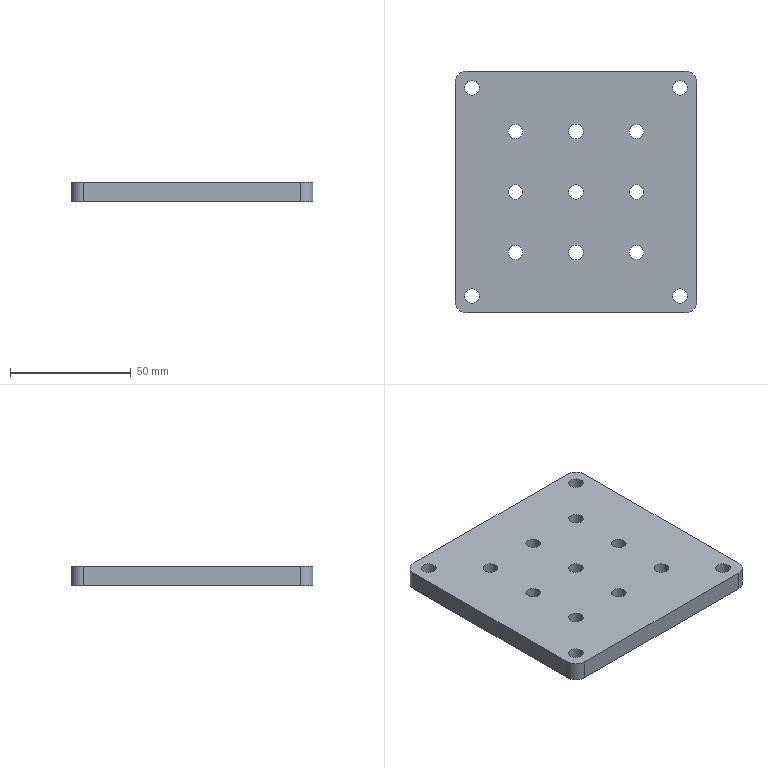Part | SolidWorks | features Extrusion 1 | 1 solid | 36 faces | box 100 x 100 x 8 mm | volume 76888 mm3 | cylinder 30 | plane 6 | commonest cylinder face diameters 6 x26 10 x4
STEP:
#1=CARTESIAN_POINT('',(-46.,-43.,8.));
#2=VERTEX_POINT('',#1);
#3=CARTESIAN_POINT('',(-40.,-43.,8.));
#4=VERTEX_POINT('',#3);
#5=CARTESIAN_POINT('',(-43.,-43.,8.));
#6=DIRECTION('',(0.,0.,1.));
#7=DIRECTION('',(1.,0.,0.));
#8=AXIS2_PLACEMENT_3D('',#5,#6,#7);
#9=CIRCLE('',#8,3.);
#10=EDGE_CURVE('',#2,#4,#9,.T.);
#11=ORIENTED_EDGE('',*,*,#10,.T.);
#12=CARTESIAN_POINT('',(-40.,-43.,0.));
#13=VERTEX_POINT('',#12);
#14=CARTESIAN_POINT('',(-40.,-43.,8.));
#15=DIRECTION('',(0.,0.,-1.));
#16=VECTOR('',#15,1000.);
#17=LINE('',#14,#16);
#18=EDGE_CURVE('',#4,#13,#17,.T.);
#19=ORIENTED_EDGE('',*,*,#18,.T.);
#20=CARTESIAN_POINT('',(-46.,-43.,0.));
#21=VERTEX_POINT('',#20);
#22=CARTESIAN_POINT('',(-43.,-43.,0.));
#23=DIRECTION('',(0.,0.,1.));
#24=DIRECTION('',(1.,0.,0.));
#25=AXIS2_PLACEMENT_3D('',#22,#23,#24);
#26=CIRCLE('',#25,3.);
#27=EDGE_CURVE('',#21,#13,#26,.T.);
#28=ORIENTED_EDGE('',*,*,#27,.F.);
#29=CARTESIAN_POINT('',(-46.,-43.,8.));
#30=DIRECTION('',(0.,0.,-1.));
#31=VECTOR('',#30,1000.);
#32=LINE('',#29,#31);
#33=EDGE_CURVE('',#2,#21,#32,.T.);
#34=ORIENTED_EDGE('',*,*,#33,.F.);
#35=EDGE_LOOP('',(#11,#19,#28,#34));
#36=FACE_OUTER_BOUND('',#35,.T.);
#37=CARTESIAN_POINT('',(-43.,-43.,8.));
#38=DIRECTION('',(0.,0.,-1.));
#39=DIRECTION('',(-1.,0.,0.));
#40=AXIS2_PLACEMENT_3D('',#37,#38,#39);
#41=CYLINDRICAL_SURFACE('',#40,3.);
#42=ADVANCED_FACE('',(#36),#41,.F.);
#43=CARTESIAN_POINT('',(40.,-43.,8.));
#44=VERTEX_POINT('',#43);
#45=CARTESIAN_POINT('',(46.,-43.,8.));
#46=VERTEX_POINT('',#45);
#47=CARTESIAN_POINT('',(43.,-43.,8.));
#48=DIRECTION('',(0.,0.,1.));
#49=DIRECTION('',(1.,0.,0.));
#50=AXIS2_PLACEMENT_3D('',#47,#48,#49);
#51=CIRCLE('',#50,3.);
#52=EDGE_CURVE('',#44,#46,#51,.T.);
#53=ORIENTED_EDGE('',*,*,#52,.T.);
#54=CARTESIAN_POINT('',(46.,-43.,0.));
#55=VERTEX_POINT('',#54);
#56=CARTESIAN_POINT('',(46.,-43.,8.));
#57=DIRECTION('',(0.,0.,-1.));
#58=VECTOR('',#57,1000.);
#59=LINE('',#56,#58);
#60=EDGE_CURVE('',#46,#55,#59,.T.);
#61=ORIENTED_EDGE('',*,*,#60,.T.);
#62=CARTESIAN_POINT('',(40.,-43.,0.));
#63=VERTEX_POINT('',#62);
#64=CARTESIAN_POINT('',(43.,-43.,0.));
#65=DIRECTION('',(0.,0.,1.));
#66=DIRECTION('',(1.,0.,0.));
#67=AXIS2_PLACEMENT_3D('',#64,#65,#66);
#68=CIRCLE('',#67,3.);
#69=EDGE_CURVE('',#63,#55,#68,.T.);
#70=ORIENTED_EDGE('',*,*,#69,.F.);
#71=CARTESIAN_POINT('',(40.,-43.,8.));
#72=DIRECTION('',(0.,0.,-1.));
#73=VECTOR('',#72,1000.);
#74=LINE('',#71,#73);
#75=EDGE_CURVE('',#44,#63,#74,.T.);
#76=ORIENTED_EDGE('',*,*,#75,.F.);
#77=EDGE_LOOP('',(#53,#61,#70,#76));
#78=FACE_OUTER_BOUND('',#77,.T.);
#79=CARTESIAN_POINT('',(43.,-43.,8.));
#80=DIRECTION('',(0.,0.,-1.));
#81=DIRECTION('',(-1.,0.,0.));
#82=AXIS2_PLACEMENT_3D('',#79,#80,#81);
#83=CYLINDRICAL_SURFACE('',#82,3.);
#84=ADVANCED_FACE('',(#78),#83,.F.);
#85=CARTESIAN_POINT('',(40.,43.,8.));
#86=VERTEX_POINT('',#85);
#87=CARTESIAN_POINT('',(46.,43.,8.));
#88=VERTEX_POINT('',#87);
#89=CARTESIAN_POINT('',(43.,43.,8.));
#90=DIRECTION('',(0.,0.,1.));
#91=DIRECTION('',(1.,0.,0.));
#92=AXIS2_PLACEMENT_3D('',#89,#90,#91);
#93=CIRCLE('',#92,3.);
#94=EDGE_CURVE('',#86,#88,#93,.T.);
#95=ORIENTED_EDGE('',*,*,#94,.T.);
#96=CARTESIAN_POINT('',(46.,43.,0.));
#97=VERTEX_POINT('',#96);
#98=CARTESIAN_POINT('',(46.,43.,8.));
#99=DIRECTION('',(0.,0.,-1.));
#100=VECTOR('',#99,1000.);
#101=LINE('',#98,#100);
#102=EDGE_CURVE('',#88,#97,#101,.T.);
#103=ORIENTED_EDGE('',*,*,#102,.T.);
#104=CARTESIAN_POINT('',(40.,43.,0.));
#105=VERTEX_POINT('',#104);
#106=CARTESIAN_POINT('',(43.,43.,0.));
#107=DIRECTION('',(0.,0.,1.));
#108=DIRECTION('',(1.,0.,0.));
#109=AXIS2_PLACEMENT_3D('',#106,#107,#108);
#110=CIRCLE('',#109,3.);
#111=EDGE_CURVE('',#105,#97,#110,.T.);
#112=ORIENTED_EDGE('',*,*,#111,.F.);
#113=CARTESIAN_POINT('',(40.,43.,8.));
#114=DIRECTION('',(0.,0.,-1.));
#115=VECTOR('',#114,1000.);
#116=LINE('',#113,#115);
#117=EDGE_CURVE('',#86,#105,#116,.T.);
#118=ORIENTED_EDGE('',*,*,#117,.F.);
#119=EDGE_LOOP('',(#95,#103,#112,#118));
#120=FACE_OUTER_BOUND('',#119,.T.);
#121=CARTESIAN_POINT('',(43.,43.,8.));
#122=DIRECTION('',(0.,0.,-1.));
#123=DIRECTION('',(-1.,0.,0.));
#124=AXIS2_PLACEMENT_3D('',#121,#122,#123);
#125=CYLINDRICAL_SURFACE('',#124,3.);
#126=ADVANCED_FACE('',(#120),#125,.F.);
#127=CARTESIAN_POINT('',(-46.,43.,8.));
#128=VERTEX_POINT('',#127);
#129=CARTESIAN_POINT('',(-40.,43.,8.));
#130=VERTEX_POINT('',#129);
#131=CARTESIAN_POINT('',(-43.,43.,8.));
#132=DIRECTION('',(0.,0.,1.));
#133=DIRECTION('',(1.,0.,0.));
#134=AXIS2_PLACEMENT_3D('',#131,#132,#133);
#135=CIRCLE('',#134,3.);
#136=EDGE_CURVE('',#128,#130,#135,.T.);
#137=ORIENTED_EDGE('',*,*,#136,.T.);
#138=CARTESIAN_POINT('',(-40.,43.,0.));
#139=VERTEX_POINT('',#138);
#140=CARTESIAN_POINT('',(-40.,43.,8.));
#141=DIRECTION('',(0.,0.,-1.));
#142=VECTOR('',#141,1000.);
#143=LINE('',#140,#142);
#144=EDGE_CURVE('',#130,#139,#143,.T.);
#145=ORIENTED_EDGE('',*,*,#144,.T.);
#146=CARTESIAN_POINT('',(-46.,43.,0.));
#147=VERTEX_POINT('',#146);
#148=CARTESIAN_POINT('',(-43.,43.,0.));
#149=DIRECTION('',(0.,0.,1.));
#150=DIRECTION('',(1.,0.,0.));
#151=AXIS2_PLACEMENT_3D('',#148,#149,#150);
#152=CIRCLE('',#151,3.);
#153=EDGE_CURVE('',#147,#139,#152,.T.);
#154=ORIENTED_EDGE('',*,*,#153,.F.);
#155=CARTESIAN_POINT('',(-46.,43.,8.));
#156=DIRECTION('',(0.,0.,-1.));
#157=VECTOR('',#156,1000.);
#158=LINE('',#155,#157);
#159=EDGE_CURVE('',#128,#147,#158,.T.);
#160=ORIENTED_EDGE('',*,*,#159,.F.);
#161=EDGE_LOOP('',(#137,#145,#154,#160));
#162=FACE_OUTER_BOUND('',#161,.T.);
#163=CARTESIAN_POINT('',(-43.,43.,8.));
#164=DIRECTION('',(0.,0.,-1.));
#165=DIRECTION('',(-1.,0.,0.));
#166=AXIS2_PLACEMENT_3D('',#163,#164,#165);
#167=CYLINDRICAL_SURFACE('',#166,3.);
#168=ADVANCED_FACE('',(#162),#167,.F.);
#169=CARTESIAN_POINT('',(-28.,-25.,8.));
#170=VERTEX_POINT('',#169);
#171=CARTESIAN_POINT('',(-22.,-25.,8.));
#172=VERTEX_POINT('',#171);
#173=CARTESIAN_POINT('',(-25.,-25.,8.));
#174=DIRECTION('',(0.,0.,1.));
#175=DIRECTION('',(1.,0.,0.));
#176=AXIS2_PLACEMENT_3D('',#173,#174,#175);
#177=CIRCLE('',#176,3.);
#178=EDGE_CURVE('',#170,#172,#177,.T.);
#179=ORIENTED_EDGE('',*,*,#178,.T.);
#180=CARTESIAN_POINT('',(-22.,-25.,0.));
#181=VERTEX_POINT('',#180);
#182=CARTESIAN_POINT('',(-22.,-25.,8.));
#183=DIRECTION('',(0.,0.,-1.));
#184=VECTOR('',#183,1000.);
#185=LINE('',#182,#184);
#186=EDGE_CURVE('',#172,#181,#185,.T.);
#187=ORIENTED_EDGE('',*,*,#186,.T.);
#188=CARTESIAN_POINT('',(-28.,-25.,0.));
#189=VERTEX_POINT('',#188);
#190=CARTESIAN_POINT('',(-25.,-25.,0.));
#191=DIRECTION('',(0.,0.,1.));
#192=DIRECTION('',(1.,0.,0.));
#193=AXIS2_PLACEMENT_3D('',#190,#191,#192);
#194=CIRCLE('',#193,3.);
#195=EDGE_CURVE('',#189,#181,#194,.T.);
#196=ORIENTED_EDGE('',*,*,#195,.F.);
#197=CARTESIAN_POINT('',(-28.,-25.,8.));
#198=DIRECTION('',(0.,0.,-1.));
#199=VECTOR('',#198,1000.);
#200=LINE('',#197,#199);
#201=EDGE_CURVE('',#170,#189,#200,.T.);
#202=ORIENTED_EDGE('',*,*,#201,.F.);
#203=EDGE_LOOP('',(#179,#187,#196,#202));
#204=FACE_OUTER_BOUND('',#203,.T.);
#205=CARTESIAN_POINT('',(-25.,-25.,8.));
#206=DIRECTION('',(0.,0.,-1.));
#207=DIRECTION('',(-1.,0.,0.));
#208=AXIS2_PLACEMENT_3D('',#205,#206,#207);
#209=CYLINDRICAL_SURFACE('',#208,3.);
#210=ADVANCED_FACE('',(#204),#209,.F.);
#211=CARTESIAN_POINT('',(-28.,0.,8.));
#212=VERTEX_POINT('',#211);
#213=CARTESIAN_POINT('',(-22.,0.,8.));
#214=VERTEX_POINT('',#213);
#215=CARTESIAN_POINT('',(-25.,0.,8.));
#216=DIRECTION('',(0.,0.,1.));
#217=DIRECTION('',(1.,0.,0.));
#218=AXIS2_PLACEMENT_3D('',#215,#216,#217);
#219=CIRCLE('',#218,3.);
#220=EDGE_CURVE('',#212,#214,#219,.T.);
#221=ORIENTED_EDGE('',*,*,#220,.T.);
#222=CARTESIAN_POINT('',(-22.,0.,0.));
#223=VERTEX_POINT('',#222);
#224=CARTESIAN_POINT('',(-22.,0.,8.));
#225=DIRECTION('',(0.,0.,-1.));
#226=VECTOR('',#225,1000.);
#227=LINE('',#224,#226);
#228=EDGE_CURVE('',#214,#223,#227,.T.);
#229=ORIENTED_EDGE('',*,*,#228,.T.);
#230=CARTESIAN_POINT('',(-28.,0.,0.));
#231=VERTEX_POINT('',#230);
#232=CARTESIAN_POINT('',(-25.,0.,0.));
#233=DIRECTION('',(0.,0.,1.));
#234=DIRECTION('',(1.,0.,0.));
#235=AXIS2_PLACEMENT_3D('',#232,#233,#234);
#236=CIRCLE('',#235,3.);
#237=EDGE_CURVE('',#231,#223,#236,.T.);
#238=ORIENTED_EDGE('',*,*,#237,.F.);
#239=CARTESIAN_POINT('',(-28.,0.,8.));
#240=DIRECTION('',(0.,0.,-1.));
#241=VECTOR('',#240,1000.);
#242=LINE('',#239,#241);
#243=EDGE_CURVE('',#212,#231,#242,.T.);
#244=ORIENTED_EDGE('',*,*,#243,.F.);
#245=EDGE_LOOP('',(#221,#229,#238,#244));
#246=FACE_OUTER_BOUND('',#245,.T.);
#247=CARTESIAN_POINT('',(-25.,0.,8.));
#248=DIRECTION('',(0.,0.,-1.));
#249=DIRECTION('',(-1.,0.,0.));
#250=AXIS2_PLACEMENT_3D('',#247,#248,#249);
#251=CYLINDRICAL_SURFACE('',#250,3.);
#252=ADVANCED_FACE('',(#246),#251,.F.);
#253=CARTESIAN_POINT('',(22.,-25.,8.));
#254=VERTEX_POINT('',#253);
#255=CARTESIAN_POINT('',(28.,-25.,8.));
#256=VERTEX_POINT('',#255);
#257=CARTESIAN_POINT('',(25.,-25.,8.));
#258=DIRECTION('',(0.,0.,1.));
#259=DIRECTION('',(1.,0.,0.));
#260=AXIS2_PLACEMENT_3D('',#257,#258,#259);
#261=CIRCLE('',#260,3.);
#262=EDGE_CURVE('',#254,#256,#261,.T.);
#263=ORIENTED_EDGE('',*,*,#262,.T.);
#264=CARTESIAN_POINT('',(28.,-25.,0.));
#265=VERTEX_POINT('',#264);
#266=CARTESIAN_POINT('',(28.,-25.,8.));
#267=DIRECTION('',(0.,0.,-1.));
#268=VECTOR('',#267,1000.);
#269=LINE('',#266,#268);
#270=EDGE_CURVE('',#256,#265,#269,.T.);
#271=ORIENTED_EDGE('',*,*,#270,.T.);
#272=CARTESIAN_POINT('',(22.,-25.,0.));
#273=VERTEX_POINT('',#272);
#274=CARTESIAN_POINT('',(25.,-25.,0.));
#275=DIRECTION('',(0.,0.,1.));
#276=DIRECTION('',(1.,0.,0.));
#277=AXIS2_PLACEMENT_3D('',#274,#275,#276);
#278=CIRCLE('',#277,3.);
#279=EDGE_CURVE('',#273,#265,#278,.T.);
#280=ORIENTED_EDGE('',*,*,#279,.F.);
#281=CARTESIAN_POINT('',(22.,-25.,8.));
#282=DIRECTION('',(0.,0.,-1.));
#283=VECTOR('',#282,1000.);
#284=LINE('',#281,#283);
#285=EDGE_CURVE('',#254,#273,#284,.T.);
#286=ORIENTED_EDGE('',*,*,#285,.F.);
#287=EDGE_LOOP('',(#263,#271,#280,#286));
#288=FACE_OUTER_BOUND('',#287,.T.);
#289=CARTESIAN_POINT('',(25.,-25.,8.));
#290=DIRECTION('',(0.,0.,-1.));
#291=DIRECTION('',(-1.,0.,0.));
#292=AXIS2_PLACEMENT_3D('',#289,#290,#291);
#293=CYLINDRICAL_SURFACE('',#292,3.);
#294=ADVANCED_FACE('',(#288),#293,.F.);
#295=CARTESIAN_POINT('',(-3.,-25.,8.));
#296=VERTEX_POINT('',#295);
#297=CARTESIAN_POINT('',(3.,-25.,8.));
#298=VERTEX_POINT('',#297);
#299=CARTESIAN_POINT('',(0.,-25.,8.));
#300=DIRECTION('',(0.,0.,1.));
#301=DIRECTION('',(1.,0.,0.));
#302=AXIS2_PLACEMENT_3D('',#299,#300,#301);
#303=CIRCLE('',#302,3.);
#304=EDGE_CURVE('',#296,#298,#303,.T.);
#305=ORIENTED_EDGE('',*,*,#304,.T.);
#306=CARTESIAN_POINT('',(3.,-25.,0.));
#307=VERTEX_POINT('',#306);
#308=CARTESIAN_POINT('',(3.,-25.,8.));
#309=DIRECTION('',(0.,0.,-1.));
#310=VECTOR('',#309,1000.);
#311=LINE('',#308,#310);
#312=EDGE_CURVE('',#298,#307,#311,.T.);
#313=ORIENTED_EDGE('',*,*,#312,.T.);
#314=CARTESIAN_POINT('',(-3.,-25.,0.));
#315=VERTEX_POINT('',#314);
#316=CARTESIAN_POINT('',(0.,-25.,0.));
#317=DIRECTION('',(0.,0.,1.));
#318=DIRECTION('',(1.,0.,0.));
#319=AXIS2_PLACEMENT_3D('',#316,#317,#318);
#320=CIRCLE('',#319,3.);
#321=EDGE_CURVE('',#315,#307,#320,.T.);
#322=ORIENTED_EDGE('',*,*,#321,.F.);
#323=CARTESIAN_POINT('',(-3.,-25.,8.));
#324=DIRECTION('',(0.,0.,-1.));
#325=VECTOR('',#324,1000.);
#326=LINE('',#323,#325);
#327=EDGE_CURVE('',#296,#315,#326,.T.);
#328=ORIENTED_EDGE('',*,*,#327,.F.);
#329=EDGE_LOOP('',(#305,#313,#322,#328));
#330=FACE_OUTER_BOUND('',#329,.T.);
#331=CARTESIAN_POINT('',(0.,-25.,8.));
#332=DIRECTION('',(0.,0.,-1.));
#333=DIRECTION('',(-1.,0.,0.));
#334=AXIS2_PLACEMENT_3D('',#331,#332,#333);
#335=CYLINDRICAL_SURFACE('',#334,3.);
#336=ADVANCED_FACE('',(#330),#335,.F.);
#337=CARTESIAN_POINT('',(22.,0.,8.));
#338=VERTEX_POINT('',#337);
#339=CARTESIAN_POINT('',(28.,0.,8.));
#340=VERTEX_POINT('',#339);
#341=CARTESIAN_POINT('',(25.,0.,8.));
#342=DIRECTION('',(0.,0.,1.));
#343=DIRECTION('',(1.,0.,0.));
#344=AXIS2_PLACEMENT_3D('',#341,#342,#343);
#345=CIRCLE('',#344,3.);
#346=EDGE_CURVE('',#338,#340,#345,.T.);
#347=ORIENTED_EDGE('',*,*,#346,.T.);
#348=CARTESIAN_POINT('',(28.,0.,0.));
#349=VERTEX_POINT('',#348);
#350=CARTESIAN_POINT('',(28.,0.,8.));
#351=DIRECTION('',(0.,0.,-1.));
#352=VECTOR('',#351,1000.);
#353=LINE('',#350,#352);
#354=EDGE_CURVE('',#340,#349,#353,.T.);
#355=ORIENTED_EDGE('',*,*,#354,.T.);
#356=CARTESIAN_POINT('',(22.,0.,0.));
#357=VERTEX_POINT('',#356);
#358=CARTESIAN_POINT('',(25.,0.,0.));
#359=DIRECTION('',(0.,0.,1.));
#360=DIRECTION('',(1.,0.,0.));
#361=AXIS2_PLACEMENT_3D('',#358,#359,#360);
#362=CIRCLE('',#361,3.);
#363=EDGE_CURVE('',#357,#349,#362,.T.);
#364=ORIENTED_EDGE('',*,*,#363,.F.);
#365=CARTESIAN_POINT('',(22.,0.,8.));
#366=DIRECTION('',(0.,0.,-1.));
#367=VECTOR('',#366,1000.);
#368=LINE('',#365,#367);
#369=EDGE_CURVE('',#338,#357,#368,.T.);
#370=ORIENTED_EDGE('',*,*,#369,.F.);
#371=EDGE_LOOP('',(#347,#355,#364,#370));
#372=FACE_OUTER_BOUND('',#371,.T.);
#373=CARTESIAN_POINT('',(25.,0.,8.));
#374=DIRECTION('',(0.,0.,-1.));
#375=DIRECTION('',(-1.,0.,0.));
#376=AXIS2_PLACEMENT_3D('',#373,#374,#375);
#377=CYLINDRICAL_SURFACE('',#376,3.);
#378=ADVANCED_FACE('',(#372),#377,.F.);
#379=CARTESIAN_POINT('',(-3.,0.,8.));
#380=VERTEX_POINT('',#379);
#381=CARTESIAN_POINT('',(3.,0.,8.));
#382=VERTEX_POINT('',#381);
#383=CARTESIAN_POINT('',(0.,0.,8.));
#384=DIRECTION('',(0.,0.,1.));
#385=DIRECTION('',(1.,0.,0.));
#386=AXIS2_PLACEMENT_3D('',#383,#384,#385);
#387=CIRCLE('',#386,3.);
#388=EDGE_CURVE('',#380,#382,#387,.T.);
#389=ORIENTED_EDGE('',*,*,#388,.T.);
#390=CARTESIAN_POINT('',(3.,0.,0.));
#391=VERTEX_POINT('',#390);
#392=CARTESIAN_POINT('',(3.,0.,8.));
#393=DIRECTION('',(0.,0.,-1.));
#394=VECTOR('',#393,1000.);
#395=LINE('',#392,#394);
#396=EDGE_CURVE('',#382,#391,#395,.T.);
#397=ORIENTED_EDGE('',*,*,#396,.T.);
#398=CARTESIAN_POINT('',(-3.,0.,0.));
#399=VERTEX_POINT('',#398);
#400=CARTESIAN_POINT('',(0.,0.,0.));
#401=DIRECTION('',(0.,0.,1.));
#402=DIRECTION('',(1.,0.,0.));
#403=AXIS2_PLACEMENT_3D('',#400,#401,#402);
#404=CIRCLE('',#403,3.);
#405=EDGE_CURVE('',#399,#391,#404,.T.);
#406=ORIENTED_EDGE('',*,*,#405,.F.);
#407=CARTESIAN_POINT('',(-3.,0.,8.));
#408=DIRECTION('',(0.,0.,-1.));
#409=VECTOR('',#408,1000.);
#410=LINE('',#407,#409);
#411=EDGE_CURVE('',#380,#399,#410,.T.);
#412=ORIENTED_EDGE('',*,*,#411,.F.);
#413=EDGE_LOOP('',(#389,#397,#406,#412));
#414=FACE_OUTER_BOUND('',#413,.T.);
#415=CARTESIAN_POINT('',(0.,0.,8.));
#416=DIRECTION('',(0.,0.,-1.));
#417=DIRECTION('',(-1.,0.,0.));
#418=AXIS2_PLACEMENT_3D('',#415,#416,#417);
#419=CYLINDRICAL_SURFACE('',#418,3.);
#420=ADVANCED_FACE('',(#414),#419,.F.);
#421=CARTESIAN_POINT('',(22.,25.,8.));
#422=VERTEX_POINT('',#421);
#423=CARTESIAN_POINT('',(28.,25.,8.));
#424=VERTEX_POINT('',#423);
#425=CARTESIAN_POINT('',(25.,25.,8.));
#426=DIRECTION('',(0.,0.,1.));
#427=DIRECTION('',(1.,0.,0.));
#428=AXIS2_PLACEMENT_3D('',#425,#426,#427);
#429=CIRCLE('',#428,3.);
#430=EDGE_CURVE('',#422,#424,#429,.T.);
#431=ORIENTED_EDGE('',*,*,#430,.T.);
#432=CARTESIAN_POINT('',(28.,25.,0.));
#433=VERTEX_POINT('',#432);
#434=CARTESIAN_POINT('',(28.,25.,8.));
#435=DIRECTION('',(0.,0.,-1.));
#436=VECTOR('',#435,1000.);
#437=LINE('',#434,#436);
#438=EDGE_CURVE('',#424,#433,#437,.T.);
#439=ORIENTED_EDGE('',*,*,#438,.T.);
#440=CARTESIAN_POINT('',(22.,25.,0.));
#441=VERTEX_POINT('',#440);
#442=CARTESIAN_POINT('',(25.,25.,0.));
#443=DIRECTION('',(0.,0.,1.));
#444=DIRECTION('',(1.,0.,0.));
#445=AXIS2_PLACEMENT_3D('',#442,#443,#444);
#446=CIRCLE('',#445,3.);
#447=EDGE_CURVE('',#441,#433,#446,.T.);
#448=ORIENTED_EDGE('',*,*,#447,.F.);
#449=CARTESIAN_POINT('',(22.,25.,8.));
#450=DIRECTION('',(0.,0.,-1.));
#451=VECTOR('',#450,1000.);
#452=LINE('',#449,#451);
#453=EDGE_CURVE('',#422,#441,#452,.T.);
#454=ORIENTED_EDGE('',*,*,#453,.F.);
#455=EDGE_LOOP('',(#431,#439,#448,#454));
#456=FACE_OUTER_BOUND('',#455,.T.);
#457=CARTESIAN_POINT('',(25.,25.,8.));
#458=DIRECTION('',(0.,0.,-1.));
#459=DIRECTION('',(-1.,0.,0.));
#460=AXIS2_PLACEMENT_3D('',#457,#458,#459);
#461=CYLINDRICAL_SURFACE('',#460,3.);
#462=ADVANCED_FACE('',(#456),#461,.F.);
#463=CARTESIAN_POINT('',(-3.,25.,8.));
#464=VERTEX_POINT('',#463);
#465=CARTESIAN_POINT('',(3.,25.,8.));
#466=VERTEX_POINT('',#465);
#467=CARTESIAN_POINT('',(0.,25.,8.));
#468=DIRECTION('',(0.,0.,1.));
#469=DIRECTION('',(1.,0.,0.));
#470=AXIS2_PLACEMENT_3D('',#467,#468,#469);
#471=CIRCLE('',#470,3.);
#472=EDGE_CURVE('',#464,#466,#471,.T.);
#473=ORIENTED_EDGE('',*,*,#472,.T.);
#474=CARTESIAN_POINT('',(3.,25.,0.));
#475=VERTEX_POINT('',#474);
#476=CARTESIAN_POINT('',(3.,25.,8.));
#477=DIRECTION('',(0.,0.,-1.));
#478=VECTOR('',#477,1000.);
#479=LINE('',#476,#478);
#480=EDGE_CURVE('',#466,#475,#479,.T.);
#481=ORIENTED_EDGE('',*,*,#480,.T.);
#482=CARTESIAN_POINT('',(-3.,25.,0.));
#483=VERTEX_POINT('',#482);
#484=CARTESIAN_POINT('',(0.,25.,0.));
#485=DIRECTION('',(0.,0.,1.));
#486=DIRECTION('',(1.,0.,0.));
#487=AXIS2_PLACEMENT_3D('',#484,#485,#486);
#488=CIRCLE('',#487,3.);
#489=EDGE_CURVE('',#483,#475,#488,.T.);
#490=ORIENTED_EDGE('',*,*,#489,.F.);
#491=CARTESIAN_POINT('',(-3.,25.,8.));
#492=DIRECTION('',(0.,0.,-1.));
#493=VECTOR('',#492,1000.);
#494=LINE('',#491,#493);
#495=EDGE_CURVE('',#464,#483,#494,.T.);
#496=ORIENTED_EDGE('',*,*,#495,.F.);
#497=EDGE_LOOP('',(#473,#481,#490,#496));
#498=FACE_OUTER_BOUND('',#497,.T.);
#499=CARTESIAN_POINT('',(0.,25.,8.));
#500=DIRECTION('',(0.,0.,-1.));
#501=DIRECTION('',(-1.,0.,0.));
#502=AXIS2_PLACEMENT_3D('',#499,#500,#501);
#503=CYLINDRICAL_SURFACE('',#502,3.);
#504=ADVANCED_FACE('',(#498),#503,.F.);
#505=CARTESIAN_POINT('',(-28.,25.,8.));
#506=VERTEX_POINT('',#505);
#507=CARTESIAN_POINT('',(-22.,25.,8.));
#508=VERTEX_POINT('',#507);
#509=CARTESIAN_POINT('',(-25.,25.,8.));
#510=DIRECTION('',(0.,0.,1.));
#511=DIRECTION('',(1.,0.,0.));
#512=AXIS2_PLACEMENT_3D('',#509,#510,#511);
#513=CIRCLE('',#512,3.);
#514=EDGE_CURVE('',#506,#508,#513,.T.);
#515=ORIENTED_EDGE('',*,*,#514,.T.);
#516=CARTESIAN_POINT('',(-22.,25.,0.));
#517=VERTEX_POINT('',#516);
#518=CARTESIAN_POINT('',(-22.,25.,8.));
#519=DIRECTION('',(0.,0.,-1.));
#520=VECTOR('',#519,1000.);
#521=LINE('',#518,#520);
#522=EDGE_CURVE('',#508,#517,#521,.T.);
#523=ORIENTED_EDGE('',*,*,#522,.T.);
#524=CARTESIAN_POINT('',(-28.,25.,0.));
#525=VERTEX_POINT('',#524);
#526=CARTESIAN_POINT('',(-25.,25.,0.));
#527=DIRECTION('',(0.,0.,1.));
#528=DIRECTION('',(1.,0.,0.));
#529=AXIS2_PLACEMENT_3D('',#526,#527,#528);
#530=CIRCLE('',#529,3.);
#531=EDGE_CURVE('',#525,#517,#530,.T.);
#532=ORIENTED_EDGE('',*,*,#531,.F.);
#533=CARTESIAN_POINT('',(-28.,25.,8.));
#534=DIRECTION('',(0.,0.,-1.));
#535=VECTOR('',#534,1000.);
#536=LINE('',#533,#535);
#537=EDGE_CURVE('',#506,#525,#536,.T.);
#538=ORIENTED_EDGE('',*,*,#537,.F.);
#539=EDGE_LOOP('',(#515,#523,#532,#538));
#540=FACE_OUTER_BOUND('',#539,.T.);
#541=CARTESIAN_POINT('',(-25.,25.,8.));
#542=DIRECTION('',(0.,0.,-1.));
#543=DIRECTION('',(-1.,0.,0.));
#544=AXIS2_PLACEMENT_3D('',#541,#542,#543);
#545=CYLINDRICAL_SURFACE('',#544,3.);
#546=ADVANCED_FACE('',(#540),#545,.F.);
#547=ORIENTED_EDGE('',*,*,#52,.F.);
#548=CARTESIAN_POINT('',(43.,-43.,8.));
#549=DIRECTION('',(0.,0.,1.));
#550=DIRECTION('',(1.,0.,0.));
#551=AXIS2_PLACEMENT_3D('',#548,#549,#550);
#552=CIRCLE('',#551,3.);
#553=EDGE_CURVE('',#46,#44,#552,.T.);
#554=ORIENTED_EDGE('',*,*,#553,.F.);
#555=EDGE_LOOP('',(#547,#554));
#556=FACE_BOUND('',#555,.T.);
#557=ORIENTED_EDGE('',*,*,#136,.F.);
#558=CARTESIAN_POINT('',(-43.,43.,8.));
#559=DIRECTION('',(0.,0.,1.));
#560=DIRECTION('',(1.,0.,0.));
#561=AXIS2_PLACEMENT_3D('',#558,#559,#560);
#562=CIRCLE('',#561,3.);
#563=EDGE_CURVE('',#130,#128,#562,.T.);
#564=ORIENTED_EDGE('',*,*,#563,.F.);
#565=EDGE_LOOP('',(#557,#564));
#566=FACE_BOUND('',#565,.T.);
#567=ORIENTED_EDGE('',*,*,#220,.F.);
#568=CARTESIAN_POINT('',(-25.,0.,8.));
#569=DIRECTION('',(0.,0.,1.));
#570=DIRECTION('',(1.,0.,0.));
#571=AXIS2_PLACEMENT_3D('',#568,#569,#570);
#572=CIRCLE('',#571,3.);
#573=EDGE_CURVE('',#214,#212,#572,.T.);
#574=ORIENTED_EDGE('',*,*,#573,.F.);
#575=EDGE_LOOP('',(#567,#574));
#576=FACE_BOUND('',#575,.T.);
#577=ORIENTED_EDGE('',*,*,#304,.F.);
#578=CARTESIAN_POINT('',(0.,-25.,8.));
#579=DIRECTION('',(0.,0.,1.));
#580=DIRECTION('',(1.,0.,0.));
#581=AXIS2_PLACEMENT_3D('',#578,#579,#580);
#582=CIRCLE('',#581,3.);
#583=EDGE_CURVE('',#298,#296,#582,.T.);
#584=ORIENTED_EDGE('',*,*,#583,.F.);
#585=EDGE_LOOP('',(#577,#584));
#586=FACE_BOUND('',#585,.T.);
#587=ORIENTED_EDGE('',*,*,#388,.F.);
#588=CARTESIAN_POINT('',(0.,0.,8.));
#589=DIRECTION('',(0.,0.,1.));
#590=DIRECTION('',(1.,0.,0.));
#591=AXIS2_PLACEMENT_3D('',#588,#589,#590);
#592=CIRCLE('',#591,3.);
#593=EDGE_CURVE('',#382,#380,#592,.T.);
#594=ORIENTED_EDGE('',*,*,#593,.F.);
#595=EDGE_LOOP('',(#587,#594));
#596=FACE_BOUND('',#595,.T.);
#597=ORIENTED_EDGE('',*,*,#472,.F.);
#598=CARTESIAN_POINT('',(0.,25.,8.));
#599=DIRECTION('',(0.,0.,1.));
#600=DIRECTION('',(1.,0.,0.));
#601=AXIS2_PLACEMENT_3D('',#598,#599,#600);
#602=CIRCLE('',#601,3.);
#603=EDGE_CURVE('',#466,#464,#602,.T.);
#604=ORIENTED_EDGE('',*,*,#603,.F.);
#605=EDGE_LOOP('',(#597,#604));
#606=FACE_BOUND('',#605,.T.);
#607=CARTESIAN_POINT('',(45.,-50.,8.));
#608=VERTEX_POINT('',#607);
#609=CARTESIAN_POINT('',(50.,-45.,8.));
#610=VERTEX_POINT('',#609);
#611=CARTESIAN_POINT('',(45.,-45.,8.));
#612=DIRECTION('',(0.,0.,1.));
#613=DIRECTION('',(1.,0.,0.));
#614=AXIS2_PLACEMENT_3D('',#611,#612,#613);
#615=CIRCLE('',#614,5.);
#616=EDGE_CURVE('',#608,#610,#615,.T.);
#617=ORIENTED_EDGE('',*,*,#616,.T.);
#618=CARTESIAN_POINT('',(50.,45.,8.));
#619=VERTEX_POINT('',#618);
#620=CARTESIAN_POINT('',(50.,45.,8.));
#621=DIRECTION('',(0.,1.,0.));
#622=VECTOR('',#621,1000.);
#623=LINE('',#620,#622);
#624=EDGE_CURVE('',#610,#619,#623,.T.);
#625=ORIENTED_EDGE('',*,*,#624,.T.);
#626=CARTESIAN_POINT('',(45.,50.,8.));
#627=VERTEX_POINT('',#626);
#628=CARTESIAN_POINT('',(45.,45.,8.));
#629=DIRECTION('',(0.,0.,1.));
#630=DIRECTION('',(-1.,0.,0.));
#631=AXIS2_PLACEMENT_3D('',#628,#629,#630);
#632=CIRCLE('',#631,5.);
#633=EDGE_CURVE('',#619,#627,#632,.T.);
#634=ORIENTED_EDGE('',*,*,#633,.T.);
#635=CARTESIAN_POINT('',(-45.,50.,8.));
#636=VERTEX_POINT('',#635);
#637=CARTESIAN_POINT('',(-45.,50.,8.));
#638=DIRECTION('',(-1.,0.,0.));
#639=VECTOR('',#638,1000.);
#640=LINE('',#637,#639);
#641=EDGE_CURVE('',#627,#636,#640,.T.);
#642=ORIENTED_EDGE('',*,*,#641,.T.);
#643=CARTESIAN_POINT('',(-50.,45.,8.));
#644=VERTEX_POINT('',#643);
#645=CARTESIAN_POINT('',(-45.,45.,8.));
#646=DIRECTION('',(0.,0.,1.));
#647=DIRECTION('',(1.,0.,0.));
#648=AXIS2_PLACEMENT_3D('',#645,#646,#647);
#649=CIRCLE('',#648,5.);
#650=EDGE_CURVE('',#636,#644,#649,.T.);
#651=ORIENTED_EDGE('',*,*,#650,.T.);
#652=CARTESIAN_POINT('',(-50.,-45.,8.));
#653=VERTEX_POINT('',#652);
#654=CARTESIAN_POINT('',(-50.,45.,8.));
#655=DIRECTION('',(0.,-1.,0.));
#656=VECTOR('',#655,1000.);
#657=LINE('',#654,#656);
#658=EDGE_CURVE('',#644,#653,#657,.T.);
#659=ORIENTED_EDGE('',*,*,#658,.T.);
#660=CARTESIAN_POINT('',(-45.,-50.,8.));
#661=VERTEX_POINT('',#660);
#662=CARTESIAN_POINT('',(-45.,-45.,8.));
#663=DIRECTION('',(0.,0.,1.));
#664=DIRECTION('',(1.,0.,0.));
#665=AXIS2_PLACEMENT_3D('',#662,#663,#664);
#666=CIRCLE('',#665,5.);
#667=EDGE_CURVE('',#653,#661,#666,.T.);
#668=ORIENTED_EDGE('',*,*,#667,.T.);
#669=CARTESIAN_POINT('',(-45.,-50.,8.));
#670=DIRECTION('',(1.,0.,0.));
#671=VECTOR('',#670,1000.);
#672=LINE('',#669,#671);
#673=EDGE_CURVE('',#661,#608,#672,.T.);
#674=ORIENTED_EDGE('',*,*,#673,.T.);
#675=EDGE_LOOP('',(#617,#625,#634,#642,#651,#659,#668,#674));
#676=FACE_OUTER_BOUND('',#675,.T.);
#677=ORIENTED_EDGE('',*,*,#514,.F.);
#678=CARTESIAN_POINT('',(-25.,25.,8.));
#679=DIRECTION('',(0.,0.,1.));
#680=DIRECTION('',(1.,0.,0.));
#681=AXIS2_PLACEMENT_3D('',#678,#679,#680);
#682=CIRCLE('',#681,3.);
#683=EDGE_CURVE('',#508,#506,#682,.T.);
#684=ORIENTED_EDGE('',*,*,#683,.F.);
#685=EDGE_LOOP('',(#677,#684));
#686=FACE_BOUND('',#685,.T.);
#687=ORIENTED_EDGE('',*,*,#430,.F.);
#688=CARTESIAN_POINT('',(25.,25.,8.));
#689=DIRECTION('',(0.,0.,1.));
#690=DIRECTION('',(1.,0.,0.));
#691=AXIS2_PLACEMENT_3D('',#688,#689,#690);
#692=CIRCLE('',#691,3.);
#693=EDGE_CURVE('',#424,#422,#692,.T.);
#694=ORIENTED_EDGE('',*,*,#693,.F.);
#695=EDGE_LOOP('',(#687,#694));
#696=FACE_BOUND('',#695,.T.);
#697=ORIENTED_EDGE('',*,*,#346,.F.);
#698=CARTESIAN_POINT('',(25.,0.,8.));
#699=DIRECTION('',(0.,0.,1.));
#700=DIRECTION('',(1.,0.,0.));
#701=AXIS2_PLACEMENT_3D('',#698,#699,#700);
#702=CIRCLE('',#701,3.);
#703=EDGE_CURVE('',#340,#338,#702,.T.);
#704=ORIENTED_EDGE('',*,*,#703,.F.);
#705=EDGE_LOOP('',(#697,#704));
#706=FACE_BOUND('',#705,.T.);
#707=ORIENTED_EDGE('',*,*,#262,.F.);
#708=CARTESIAN_POINT('',(25.,-25.,8.));
#709=DIRECTION('',(0.,0.,1.));
#710=DIRECTION('',(1.,0.,0.));
#711=AXIS2_PLACEMENT_3D('',#708,#709,#710);
#712=CIRCLE('',#711,3.);
#713=EDGE_CURVE('',#256,#254,#712,.T.);
#714=ORIENTED_EDGE('',*,*,#713,.F.);
#715=EDGE_LOOP('',(#707,#714));
#716=FACE_BOUND('',#715,.T.);
#717=ORIENTED_EDGE('',*,*,#178,.F.);
#718=CARTESIAN_POINT('',(-25.,-25.,8.));
#719=DIRECTION('',(0.,0.,1.));
#720=DIRECTION('',(1.,0.,0.));
#721=AXIS2_PLACEMENT_3D('',#718,#719,#720);
#722=CIRCLE('',#721,3.);
#723=EDGE_CURVE('',#172,#170,#722,.T.);
#724=ORIENTED_EDGE('',*,*,#723,.F.);
#725=EDGE_LOOP('',(#717,#724));
#726=FACE_BOUND('',#725,.T.);
#727=ORIENTED_EDGE('',*,*,#94,.F.);
#728=CARTESIAN_POINT('',(43.,43.,8.));
#729=DIRECTION('',(0.,0.,1.));
#730=DIRECTION('',(1.,0.,0.));
#731=AXIS2_PLACEMENT_3D('',#728,#729,#730);
#732=CIRCLE('',#731,3.);
#733=EDGE_CURVE('',#88,#86,#732,.T.);
#734=ORIENTED_EDGE('',*,*,#733,.F.);
#735=EDGE_LOOP('',(#727,#734));
#736=FACE_BOUND('',#735,.T.);
#737=ORIENTED_EDGE('',*,*,#10,.F.);
#738=CARTESIAN_POINT('',(-43.,-43.,8.));
#739=DIRECTION('',(0.,0.,1.));
#740=DIRECTION('',(1.,0.,0.));
#741=AXIS2_PLACEMENT_3D('',#738,#739,#740);
#742=CIRCLE('',#741,3.);
#743=EDGE_CURVE('',#4,#2,#742,.T.);
#744=ORIENTED_EDGE('',*,*,#743,.F.);
#745=EDGE_LOOP('',(#737,#744));
#746=FACE_BOUND('',#745,.T.);
#747=CARTESIAN_POINT('',(45.,-45.,8.));
#748=DIRECTION('',(0.,0.,1.));
#749=DIRECTION('',(1.,0.,0.));
#750=AXIS2_PLACEMENT_3D('',#747,#748,#749);
#751=PLANE('',#750);
#752=ADVANCED_FACE('',(#556,#566,#576,#586,#596,#606,#676,#686,#696,#706,#716,#726,#736,#746),#751,.T.);
#753=CARTESIAN_POINT('',(45.,-50.,0.));
#754=VERTEX_POINT('',#753);
#755=CARTESIAN_POINT('',(50.,-45.,0.));
#756=VERTEX_POINT('',#755);
#757=CARTESIAN_POINT('',(45.,-45.,0.));
#758=DIRECTION('',(0.,0.,1.));
#759=DIRECTION('',(1.,0.,0.));
#760=AXIS2_PLACEMENT_3D('',#757,#758,#759);
#761=CIRCLE('',#760,5.);
#762=EDGE_CURVE('',#754,#756,#761,.T.);
#763=ORIENTED_EDGE('',*,*,#762,.F.);
#764=CARTESIAN_POINT('',(-45.,-50.,0.));
#765=VERTEX_POINT('',#764);
#766=CARTESIAN_POINT('',(-45.,-50.,0.));
#767=DIRECTION('',(1.,0.,0.));
#768=VECTOR('',#767,1000.);
#769=LINE('',#766,#768);
#770=EDGE_CURVE('',#765,#754,#769,.T.);
#771=ORIENTED_EDGE('',*,*,#770,.F.);
#772=CARTESIAN_POINT('',(-50.,-45.,0.));
#773=VERTEX_POINT('',#772);
#774=CARTESIAN_POINT('',(-45.,-45.,0.));
#775=DIRECTION('',(0.,0.,1.));
#776=DIRECTION('',(1.,0.,0.));
#777=AXIS2_PLACEMENT_3D('',#774,#775,#776);
#778=CIRCLE('',#777,5.);
#779=EDGE_CURVE('',#773,#765,#778,.T.);
#780=ORIENTED_EDGE('',*,*,#779,.F.);
#781=CARTESIAN_POINT('',(-50.,45.,0.));
#782=VERTEX_POINT('',#781);
#783=CARTESIAN_POINT('',(-50.,45.,0.));
#784=DIRECTION('',(0.,-1.,0.));
#785=VECTOR('',#784,1000.);
#786=LINE('',#783,#785);
#787=EDGE_CURVE('',#782,#773,#786,.T.);
#788=ORIENTED_EDGE('',*,*,#787,.F.);
#789=CARTESIAN_POINT('',(-45.,50.,0.));
#790=VERTEX_POINT('',#789);
#791=CARTESIAN_POINT('',(-45.,45.,0.));
#792=DIRECTION('',(0.,0.,1.));
#793=DIRECTION('',(1.,0.,0.));
#794=AXIS2_PLACEMENT_3D('',#791,#792,#793);
#795=CIRCLE('',#794,5.);
#796=EDGE_CURVE('',#790,#782,#795,.T.);
#797=ORIENTED_EDGE('',*,*,#796,.F.);
#798=CARTESIAN_POINT('',(45.,50.,0.));
#799=VERTEX_POINT('',#798);
#800=CARTESIAN_POINT('',(-45.,50.,0.));
#801=DIRECTION('',(-1.,0.,0.));
#802=VECTOR('',#801,1000.);
#803=LINE('',#800,#802);
#804=EDGE_CURVE('',#799,#790,#803,.T.);
#805=ORIENTED_EDGE('',*,*,#804,.F.);
#806=CARTESIAN_POINT('',(50.,45.,0.));
#807=VERTEX_POINT('',#806);
#808=CARTESIAN_POINT('',(45.,45.,0.));
#809=DIRECTION('',(0.,0.,1.));
#810=DIRECTION('',(-1.,0.,0.));
#811=AXIS2_PLACEMENT_3D('',#808,#809,#810);
#812=CIRCLE('',#811,5.);
#813=EDGE_CURVE('',#807,#799,#812,.T.);
#814=ORIENTED_EDGE('',*,*,#813,.F.);
#815=CARTESIAN_POINT('',(50.,45.,0.));
#816=DIRECTION('',(0.,1.,0.));
#817=VECTOR('',#816,1000.);
#818=LINE('',#815,#817);
#819=EDGE_CURVE('',#756,#807,#818,.T.);
#820=ORIENTED_EDGE('',*,*,#819,.F.);
#821=EDGE_LOOP('',(#763,#771,#780,#788,#797,#805,#814,#820));
#822=FACE_OUTER_BOUND('',#821,.T.);
#823=ORIENTED_EDGE('',*,*,#531,.T.);
#824=CARTESIAN_POINT('',(-25.,25.,0.));
#825=DIRECTION('',(0.,0.,1.));
#826=DIRECTION('',(1.,0.,0.));
#827=AXIS2_PLACEMENT_3D('',#824,#825,#826);
#828=CIRCLE('',#827,3.);
#829=EDGE_CURVE('',#517,#525,#828,.T.);
#830=ORIENTED_EDGE('',*,*,#829,.T.);
#831=EDGE_LOOP('',(#823,#830));
#832=FACE_BOUND('',#831,.T.);
#833=ORIENTED_EDGE('',*,*,#489,.T.);
#834=CARTESIAN_POINT('',(0.,25.,0.));
#835=DIRECTION('',(0.,0.,1.));
#836=DIRECTION('',(1.,0.,0.));
#837=AXIS2_PLACEMENT_3D('',#834,#835,#836);
#838=CIRCLE('',#837,3.);
#839=EDGE_CURVE('',#475,#483,#838,.T.);
#840=ORIENTED_EDGE('',*,*,#839,.T.);
#841=EDGE_LOOP('',(#833,#840));
#842=FACE_BOUND('',#841,.T.);
#843=ORIENTED_EDGE('',*,*,#447,.T.);
#844=CARTESIAN_POINT('',(25.,25.,0.));
#845=DIRECTION('',(0.,0.,1.));
#846=DIRECTION('',(1.,0.,0.));
#847=AXIS2_PLACEMENT_3D('',#844,#845,#846);
#848=CIRCLE('',#847,3.);
#849=EDGE_CURVE('',#433,#441,#848,.T.);
#850=ORIENTED_EDGE('',*,*,#849,.T.);
#851=EDGE_LOOP('',(#843,#850));
#852=FACE_BOUND('',#851,.T.);
#853=ORIENTED_EDGE('',*,*,#405,.T.);
#854=CARTESIAN_POINT('',(0.,0.,0.));
#855=DIRECTION('',(0.,0.,1.));
#856=DIRECTION('',(1.,0.,0.));
#857=AXIS2_PLACEMENT_3D('',#854,#855,#856);
#858=CIRCLE('',#857,3.);
#859=EDGE_CURVE('',#391,#399,#858,.T.);
#860=ORIENTED_EDGE('',*,*,#859,.T.);
#861=EDGE_LOOP('',(#853,#860));
#862=FACE_BOUND('',#861,.T.);
#863=ORIENTED_EDGE('',*,*,#363,.T.);
#864=CARTESIAN_POINT('',(25.,0.,0.));
#865=DIRECTION('',(0.,0.,1.));
#866=DIRECTION('',(1.,0.,0.));
#867=AXIS2_PLACEMENT_3D('',#864,#865,#866);
#868=CIRCLE('',#867,3.);
#869=EDGE_CURVE('',#349,#357,#868,.T.);
#870=ORIENTED_EDGE('',*,*,#869,.T.);
#871=EDGE_LOOP('',(#863,#870));
#872=FACE_BOUND('',#871,.T.);
#873=ORIENTED_EDGE('',*,*,#321,.T.);
#874=CARTESIAN_POINT('',(0.,-25.,0.));
#875=DIRECTION('',(0.,0.,1.));
#876=DIRECTION('',(1.,0.,0.));
#877=AXIS2_PLACEMENT_3D('',#874,#875,#876);
#878=CIRCLE('',#877,3.);
#879=EDGE_CURVE('',#307,#315,#878,.T.);
#880=ORIENTED_EDGE('',*,*,#879,.T.);
#881=EDGE_LOOP('',(#873,#880));
#882=FACE_BOUND('',#881,.T.);
#883=ORIENTED_EDGE('',*,*,#279,.T.);
#884=CARTESIAN_POINT('',(25.,-25.,0.));
#885=DIRECTION('',(0.,0.,1.));
#886=DIRECTION('',(1.,0.,0.));
#887=AXIS2_PLACEMENT_3D('',#884,#885,#886);
#888=CIRCLE('',#887,3.);
#889=EDGE_CURVE('',#265,#273,#888,.T.);
#890=ORIENTED_EDGE('',*,*,#889,.T.);
#891=EDGE_LOOP('',(#883,#890));
#892=FACE_BOUND('',#891,.T.);
#893=ORIENTED_EDGE('',*,*,#237,.T.);
#894=CARTESIAN_POINT('',(-25.,0.,0.));
#895=DIRECTION('',(0.,0.,1.));
#896=DIRECTION('',(1.,0.,0.));
#897=AXIS2_PLACEMENT_3D('',#894,#895,#896);
#898=CIRCLE('',#897,3.);
#899=EDGE_CURVE('',#223,#231,#898,.T.);
#900=ORIENTED_EDGE('',*,*,#899,.T.);
#901=EDGE_LOOP('',(#893,#900));
#902=FACE_BOUND('',#901,.T.);
#903=ORIENTED_EDGE('',*,*,#195,.T.);
#904=CARTESIAN_POINT('',(-25.,-25.,0.));
#905=DIRECTION('',(0.,0.,1.));
#906=DIRECTION('',(1.,0.,0.));
#907=AXIS2_PLACEMENT_3D('',#904,#905,#906);
#908=CIRCLE('',#907,3.);
#909=EDGE_CURVE('',#181,#189,#908,.T.);
#910=ORIENTED_EDGE('',*,*,#909,.T.);
#911=EDGE_LOOP('',(#903,#910));
#912=FACE_BOUND('',#911,.T.);
#913=ORIENTED_EDGE('',*,*,#153,.T.);
#914=CARTESIAN_POINT('',(-43.,43.,0.));
#915=DIRECTION('',(0.,0.,1.));
#916=DIRECTION('',(1.,0.,0.));
#917=AXIS2_PLACEMENT_3D('',#914,#915,#916);
#918=CIRCLE('',#917,3.);
#919=EDGE_CURVE('',#139,#147,#918,.T.);
#920=ORIENTED_EDGE('',*,*,#919,.T.);
#921=EDGE_LOOP('',(#913,#920));
#922=FACE_BOUND('',#921,.T.);
#923=ORIENTED_EDGE('',*,*,#111,.T.);
#924=CARTESIAN_POINT('',(43.,43.,0.));
#925=DIRECTION('',(0.,0.,1.));
#926=DIRECTION('',(1.,0.,0.));
#927=AXIS2_PLACEMENT_3D('',#924,#925,#926);
#928=CIRCLE('',#927,3.);
#929=EDGE_CURVE('',#97,#105,#928,.T.);
#930=ORIENTED_EDGE('',*,*,#929,.T.);
#931=EDGE_LOOP('',(#923,#930));
#932=FACE_BOUND('',#931,.T.);
#933=ORIENTED_EDGE('',*,*,#69,.T.);
#934=CARTESIAN_POINT('',(43.,-43.,0.));
#935=DIRECTION('',(0.,0.,1.));
#936=DIRECTION('',(1.,0.,0.));
#937=AXIS2_PLACEMENT_3D('',#934,#935,#936);
#938=CIRCLE('',#937,3.);
#939=EDGE_CURVE('',#55,#63,#938,.T.);
#940=ORIENTED_EDGE('',*,*,#939,.T.);
#941=EDGE_LOOP('',(#933,#940));
#942=FACE_BOUND('',#941,.T.);
#943=ORIENTED_EDGE('',*,*,#27,.T.);
#944=CARTESIAN_POINT('',(-43.,-43.,0.));
#945=DIRECTION('',(0.,0.,1.));
#946=DIRECTION('',(1.,0.,0.));
#947=AXIS2_PLACEMENT_3D('',#944,#945,#946);
#948=CIRCLE('',#947,3.);
#949=EDGE_CURVE('',#13,#21,#948,.T.);
#950=ORIENTED_EDGE('',*,*,#949,.T.);
#951=EDGE_LOOP('',(#943,#950));
#952=FACE_BOUND('',#951,.T.);
#953=CARTESIAN_POINT('',(45.,-45.,0.));
#954=DIRECTION('',(0.,0.,1.));
#955=DIRECTION('',(1.,0.,0.));
#956=AXIS2_PLACEMENT_3D('',#953,#954,#955);
#957=PLANE('',#956);
#958=ADVANCED_FACE('',(#822,#832,#842,#852,#862,#872,#882,#892,#902,#912,#922,#932,#942,#952),#957,.F.);
#959=ORIENTED_EDGE('',*,*,#762,.T.);
#960=CARTESIAN_POINT('',(50.,-45.,8.));
#961=DIRECTION('',(0.,0.,-1.));
#962=VECTOR('',#961,1000.);
#963=LINE('',#960,#962);
#964=EDGE_CURVE('',#610,#756,#963,.T.);
#965=ORIENTED_EDGE('',*,*,#964,.F.);
#966=ORIENTED_EDGE('',*,*,#616,.F.);
#967=CARTESIAN_POINT('',(45.,-50.,8.));
#968=DIRECTION('',(0.,0.,-1.));
#969=VECTOR('',#968,1000.);
#970=LINE('',#967,#969);
#971=EDGE_CURVE('',#608,#754,#970,.T.);
#972=ORIENTED_EDGE('',*,*,#971,.T.);
#973=EDGE_LOOP('',(#959,#965,#966,#972));
#974=FACE_OUTER_BOUND('',#973,.T.);
#975=CARTESIAN_POINT('',(45.,-45.,8.));
#976=DIRECTION('',(0.,0.,-1.));
#977=DIRECTION('',(-1.,0.,0.));
#978=AXIS2_PLACEMENT_3D('',#975,#976,#977);
#979=CYLINDRICAL_SURFACE('',#978,5.);
#980=ADVANCED_FACE('',(#974),#979,.T.);
#981=ORIENTED_EDGE('',*,*,#819,.T.);
#982=CARTESIAN_POINT('',(50.,45.,8.));
#983=DIRECTION('',(0.,0.,-1.));
#984=VECTOR('',#983,1000.);
#985=LINE('',#982,#984);
#986=EDGE_CURVE('',#619,#807,#985,.T.);
#987=ORIENTED_EDGE('',*,*,#986,.F.);
#988=ORIENTED_EDGE('',*,*,#624,.F.);
#989=ORIENTED_EDGE('',*,*,#964,.T.);
#990=EDGE_LOOP('',(#981,#987,#988,#989));
#991=FACE_OUTER_BOUND('',#990,.T.);
#992=CARTESIAN_POINT('',(50.,45.,8.));
#993=DIRECTION('',(-1.,0.,0.));
#994=DIRECTION('',(0.,-1.,0.));
#995=AXIS2_PLACEMENT_3D('',#992,#993,#994);
#996=PLANE('',#995);
#997=ADVANCED_FACE('',(#991),#996,.F.);
#998=ORIENTED_EDGE('',*,*,#813,.T.);
#999=CARTESIAN_POINT('',(45.,50.,8.));
#1000=DIRECTION('',(0.,0.,-1.));
#1001=VECTOR('',#1000,1000.);
#1002=LINE('',#999,#1001);
#1003=EDGE_CURVE('',#627,#799,#1002,.T.);
#1004=ORIENTED_EDGE('',*,*,#1003,.F.);
#1005=ORIENTED_EDGE('',*,*,#633,.F.);
#1006=ORIENTED_EDGE('',*,*,#986,.T.);
#1007=EDGE_LOOP('',(#998,#1004,#1005,#1006));
#1008=FACE_OUTER_BOUND('',#1007,.T.);
#1009=CARTESIAN_POINT('',(45.,45.,8.));
#1010=DIRECTION('',(0.,0.,-1.));
#1011=DIRECTION('',(-1.,0.,0.));
#1012=AXIS2_PLACEMENT_3D('',#1009,#1010,#1011);
#1013=CYLINDRICAL_SURFACE('',#1012,5.);
#1014=ADVANCED_FACE('',(#1008),#1013,.T.);
#1015=ORIENTED_EDGE('',*,*,#804,.T.);
#1016=CARTESIAN_POINT('',(-45.,50.,8.));
#1017=DIRECTION('',(0.,0.,-1.));
#1018=VECTOR('',#1017,1000.);
#1019=LINE('',#1016,#1018);
#1020=EDGE_CURVE('',#636,#790,#1019,.T.);
#1021=ORIENTED_EDGE('',*,*,#1020,.F.);
#1022=ORIENTED_EDGE('',*,*,#641,.F.);
#1023=ORIENTED_EDGE('',*,*,#1003,.T.);
#1024=EDGE_LOOP('',(#1015,#1021,#1022,#1023));
#1025=FACE_OUTER_BOUND('',#1024,.T.);
#1026=CARTESIAN_POINT('',(-45.,50.,8.));
#1027=DIRECTION('',(0.,-1.,0.));
#1028=DIRECTION('',(0.,0.,-1.));
#1029=AXIS2_PLACEMENT_3D('',#1026,#1027,#1028);
#1030=PLANE('',#1029);
#1031=ADVANCED_FACE('',(#1025),#1030,.F.);
#1032=ORIENTED_EDGE('',*,*,#796,.T.);
#1033=CARTESIAN_POINT('',(-50.,45.,8.));
#1034=DIRECTION('',(0.,0.,-1.));
#1035=VECTOR('',#1034,1000.);
#1036=LINE('',#1033,#1035);
#1037=EDGE_CURVE('',#644,#782,#1036,.T.);
#1038=ORIENTED_EDGE('',*,*,#1037,.F.);
#1039=ORIENTED_EDGE('',*,*,#650,.F.);
#1040=ORIENTED_EDGE('',*,*,#1020,.T.);
#1041=EDGE_LOOP('',(#1032,#1038,#1039,#1040));
#1042=FACE_OUTER_BOUND('',#1041,.T.);
#1043=CARTESIAN_POINT('',(-45.,45.,8.));
#1044=DIRECTION('',(0.,0.,-1.));
#1045=DIRECTION('',(-1.,0.,0.));
#1046=AXIS2_PLACEMENT_3D('',#1043,#1044,#1045);
#1047=CYLINDRICAL_SURFACE('',#1046,5.);
#1048=ADVANCED_FACE('',(#1042),#1047,.T.);
#1049=ORIENTED_EDGE('',*,*,#787,.T.);
#1050=CARTESIAN_POINT('',(-50.,-45.,8.));
#1051=DIRECTION('',(0.,0.,-1.));
#1052=VECTOR('',#1051,1000.);
#1053=LINE('',#1050,#1052);
#1054=EDGE_CURVE('',#653,#773,#1053,.T.);
#1055=ORIENTED_EDGE('',*,*,#1054,.F.);
#1056=ORIENTED_EDGE('',*,*,#658,.F.);
#1057=ORIENTED_EDGE('',*,*,#1037,.T.);
#1058=EDGE_LOOP('',(#1049,#1055,#1056,#1057));
#1059=FACE_OUTER_BOUND('',#1058,.T.);
#1060=CARTESIAN_POINT('',(-50.,45.,8.));
#1061=DIRECTION('',(1.,0.,0.));
#1062=DIRECTION('',(0.,1.,0.));
#1063=AXIS2_PLACEMENT_3D('',#1060,#1061,#1062);
#1064=PLANE('',#1063);
#1065=ADVANCED_FACE('',(#1059),#1064,.F.);
#1066=ORIENTED_EDGE('',*,*,#779,.T.);
#1067=CARTESIAN_POINT('',(-45.,-50.,8.));
#1068=DIRECTION('',(0.,0.,-1.));
#1069=VECTOR('',#1068,1000.);
#1070=LINE('',#1067,#1069);
#1071=EDGE_CURVE('',#661,#765,#1070,.T.);
#1072=ORIENTED_EDGE('',*,*,#1071,.F.);
#1073=ORIENTED_EDGE('',*,*,#667,.F.);
#1074=ORIENTED_EDGE('',*,*,#1054,.T.);
#1075=EDGE_LOOP('',(#1066,#1072,#1073,#1074));
#1076=FACE_OUTER_BOUND('',#1075,.T.);
#1077=CARTESIAN_POINT('',(-45.,-45.,8.));
#1078=DIRECTION('',(0.,0.,-1.));
#1079=DIRECTION('',(-1.,0.,0.));
#1080=AXIS2_PLACEMENT_3D('',#1077,#1078,#1079);
#1081=CYLINDRICAL_SURFACE('',#1080,5.);
#1082=ADVANCED_FACE('',(#1076),#1081,.T.);
#1083=ORIENTED_EDGE('',*,*,#770,.T.);
#1084=ORIENTED_EDGE('',*,*,#971,.F.);
#1085=ORIENTED_EDGE('',*,*,#673,.F.);
#1086=ORIENTED_EDGE('',*,*,#1071,.T.);
#1087=EDGE_LOOP('',(#1083,#1084,#1085,#1086));
#1088=FACE_OUTER_BOUND('',#1087,.T.);
#1089=CARTESIAN_POINT('',(-45.,-50.,8.));
#1090=DIRECTION('',(0.,1.,0.));
#1091=DIRECTION('',(0.,0.,1.));
#1092=AXIS2_PLACEMENT_3D('',#1089,#1090,#1091);
#1093=PLANE('',#1092);
#1094=ADVANCED_FACE('',(#1088),#1093,.F.);
#1095=ORIENTED_EDGE('',*,*,#522,.F.);
#1096=ORIENTED_EDGE('',*,*,#683,.T.);
#1097=ORIENTED_EDGE('',*,*,#537,.T.);
#1098=ORIENTED_EDGE('',*,*,#829,.F.);
#1099=EDGE_LOOP('',(#1095,#1096,#1097,#1098));
#1100=FACE_OUTER_BOUND('',#1099,.T.);
#1101=CARTESIAN_POINT('',(-25.,25.,8.));
#1102=DIRECTION('',(0.,0.,-1.));
#1103=DIRECTION('',(-1.,0.,0.));
#1104=AXIS2_PLACEMENT_3D('',#1101,#1102,#1103);
#1105=CYLINDRICAL_SURFACE('',#1104,3.);
#1106=ADVANCED_FACE('',(#1100),#1105,.F.);
#1107=ORIENTED_EDGE('',*,*,#480,.F.);
#1108=ORIENTED_EDGE('',*,*,#603,.T.);
#1109=ORIENTED_EDGE('',*,*,#495,.T.);
#1110=ORIENTED_EDGE('',*,*,#839,.F.);
#1111=EDGE_LOOP('',(#1107,#1108,#1109,#1110));
#1112=FACE_OUTER_BOUND('',#1111,.T.);
#1113=CARTESIAN_POINT('',(0.,25.,8.));
#1114=DIRECTION('',(0.,0.,-1.));
#1115=DIRECTION('',(-1.,0.,0.));
#1116=AXIS2_PLACEMENT_3D('',#1113,#1114,#1115);
#1117=CYLINDRICAL_SURFACE('',#1116,3.);
#1118=ADVANCED_FACE('',(#1112),#1117,.F.);
#1119=ORIENTED_EDGE('',*,*,#438,.F.);
#1120=ORIENTED_EDGE('',*,*,#693,.T.);
#1121=ORIENTED_EDGE('',*,*,#453,.T.);
#1122=ORIENTED_EDGE('',*,*,#849,.F.);
#1123=EDGE_LOOP('',(#1119,#1120,#1121,#1122));
#1124=FACE_OUTER_BOUND('',#1123,.T.);
#1125=CARTESIAN_POINT('',(25.,25.,8.));
#1126=DIRECTION('',(0.,0.,-1.));
#1127=DIRECTION('',(-1.,0.,0.));
#1128=AXIS2_PLACEMENT_3D('',#1125,#1126,#1127);
#1129=CYLINDRICAL_SURFACE('',#1128,3.);
#1130=ADVANCED_FACE('',(#1124),#1129,.F.);
#1131=ORIENTED_EDGE('',*,*,#396,.F.);
#1132=ORIENTED_EDGE('',*,*,#593,.T.);
#1133=ORIENTED_EDGE('',*,*,#411,.T.);
#1134=ORIENTED_EDGE('',*,*,#859,.F.);
#1135=EDGE_LOOP('',(#1131,#1132,#1133,#1134));
#1136=FACE_OUTER_BOUND('',#1135,.T.);
#1137=CARTESIAN_POINT('',(0.,0.,8.));
#1138=DIRECTION('',(0.,0.,-1.));
#1139=DIRECTION('',(-1.,0.,0.));
#1140=AXIS2_PLACEMENT_3D('',#1137,#1138,#1139);
#1141=CYLINDRICAL_SURFACE('',#1140,3.);
#1142=ADVANCED_FACE('',(#1136),#1141,.F.);
#1143=ORIENTED_EDGE('',*,*,#354,.F.);
#1144=ORIENTED_EDGE('',*,*,#703,.T.);
#1145=ORIENTED_EDGE('',*,*,#369,.T.);
#1146=ORIENTED_EDGE('',*,*,#869,.F.);
#1147=EDGE_LOOP('',(#1143,#1144,#1145,#1146));
#1148=FACE_OUTER_BOUND('',#1147,.T.);
#1149=CARTESIAN_POINT('',(25.,0.,8.));
#1150=DIRECTION('',(0.,0.,-1.));
#1151=DIRECTION('',(-1.,0.,0.));
#1152=AXIS2_PLACEMENT_3D('',#1149,#1150,#1151);
#1153=CYLINDRICAL_SURFACE('',#1152,3.);
#1154=ADVANCED_FACE('',(#1148),#1153,.F.);
#1155=ORIENTED_EDGE('',*,*,#312,.F.);
#1156=ORIENTED_EDGE('',*,*,#583,.T.);
#1157=ORIENTED_EDGE('',*,*,#327,.T.);
#1158=ORIENTED_EDGE('',*,*,#879,.F.);
#1159=EDGE_LOOP('',(#1155,#1156,#1157,#1158));
#1160=FACE_OUTER_BOUND('',#1159,.T.);
#1161=CARTESIAN_POINT('',(0.,-25.,8.));
#1162=DIRECTION('',(0.,0.,-1.));
#1163=DIRECTION('',(-1.,0.,0.));
#1164=AXIS2_PLACEMENT_3D('',#1161,#1162,#1163);
#1165=CYLINDRICAL_SURFACE('',#1164,3.);
#1166=ADVANCED_FACE('',(#1160),#1165,.F.);
#1167=ORIENTED_EDGE('',*,*,#270,.F.);
#1168=ORIENTED_EDGE('',*,*,#713,.T.);
#1169=ORIENTED_EDGE('',*,*,#285,.T.);
#1170=ORIENTED_EDGE('',*,*,#889,.F.);
#1171=EDGE_LOOP('',(#1167,#1168,#1169,#1170));
#1172=FACE_OUTER_BOUND('',#1171,.T.);
#1173=CARTESIAN_POINT('',(25.,-25.,8.));
#1174=DIRECTION('',(0.,0.,-1.));
#1175=DIRECTION('',(-1.,0.,0.));
#1176=AXIS2_PLACEMENT_3D('',#1173,#1174,#1175);
#1177=CYLINDRICAL_SURFACE('',#1176,3.);
#1178=ADVANCED_FACE('',(#1172),#1177,.F.);
#1179=ORIENTED_EDGE('',*,*,#228,.F.);
#1180=ORIENTED_EDGE('',*,*,#573,.T.);
#1181=ORIENTED_EDGE('',*,*,#243,.T.);
#1182=ORIENTED_EDGE('',*,*,#899,.F.);
#1183=EDGE_LOOP('',(#1179,#1180,#1181,#1182));
#1184=FACE_OUTER_BOUND('',#1183,.T.);
#1185=CARTESIAN_POINT('',(-25.,0.,8.));
#1186=DIRECTION('',(0.,0.,-1.));
#1187=DIRECTION('',(-1.,0.,0.));
#1188=AXIS2_PLACEMENT_3D('',#1185,#1186,#1187);
#1189=CYLINDRICAL_SURFACE('',#1188,3.);
#1190=ADVANCED_FACE('',(#1184),#1189,.F.);
#1191=ORIENTED_EDGE('',*,*,#186,.F.);
#1192=ORIENTED_EDGE('',*,*,#723,.T.);
#1193=ORIENTED_EDGE('',*,*,#201,.T.);
#1194=ORIENTED_EDGE('',*,*,#909,.F.);
#1195=EDGE_LOOP('',(#1191,#1192,#1193,#1194));
#1196=FACE_OUTER_BOUND('',#1195,.T.);
#1197=CARTESIAN_POINT('',(-25.,-25.,8.));
#1198=DIRECTION('',(0.,0.,-1.));
#1199=DIRECTION('',(-1.,0.,0.));
#1200=AXIS2_PLACEMENT_3D('',#1197,#1198,#1199);
#1201=CYLINDRICAL_SURFACE('',#1200,3.);
#1202=ADVANCED_FACE('',(#1196),#1201,.F.);
#1203=ORIENTED_EDGE('',*,*,#144,.F.);
#1204=ORIENTED_EDGE('',*,*,#563,.T.);
#1205=ORIENTED_EDGE('',*,*,#159,.T.);
#1206=ORIENTED_EDGE('',*,*,#919,.F.);
#1207=EDGE_LOOP('',(#1203,#1204,#1205,#1206));
#1208=FACE_OUTER_BOUND('',#1207,.T.);
#1209=CARTESIAN_POINT('',(-43.,43.,8.));
#1210=DIRECTION('',(0.,0.,-1.));
#1211=DIRECTION('',(-1.,0.,0.));
#1212=AXIS2_PLACEMENT_3D('',#1209,#1210,#1211);
#1213=CYLINDRICAL_SURFACE('',#1212,3.);
#1214=ADVANCED_FACE('',(#1208),#1213,.F.);
#1215=ORIENTED_EDGE('',*,*,#102,.F.);
#1216=ORIENTED_EDGE('',*,*,#733,.T.);
#1217=ORIENTED_EDGE('',*,*,#117,.T.);
#1218=ORIENTED_EDGE('',*,*,#929,.F.);
#1219=EDGE_LOOP('',(#1215,#1216,#1217,#1218));
#1220=FACE_OUTER_BOUND('',#1219,.T.);
#1221=CARTESIAN_POINT('',(43.,43.,8.));
#1222=DIRECTION('',(0.,0.,-1.));
#1223=DIRECTION('',(-1.,0.,0.));
#1224=AXIS2_PLACEMENT_3D('',#1221,#1222,#1223);
#1225=CYLINDRICAL_SURFACE('',#1224,3.);
#1226=ADVANCED_FACE('',(#1220),#1225,.F.);
#1227=ORIENTED_EDGE('',*,*,#60,.F.);
#1228=ORIENTED_EDGE('',*,*,#553,.T.);
#1229=ORIENTED_EDGE('',*,*,#75,.T.);
#1230=ORIENTED_EDGE('',*,*,#939,.F.);
#1231=EDGE_LOOP('',(#1227,#1228,#1229,#1230));
#1232=FACE_OUTER_BOUND('',#1231,.T.);
#1233=CARTESIAN_POINT('',(43.,-43.,8.));
#1234=DIRECTION('',(0.,0.,-1.));
#1235=DIRECTION('',(-1.,0.,0.));
#1236=AXIS2_PLACEMENT_3D('',#1233,#1234,#1235);
#1237=CYLINDRICAL_SURFACE('',#1236,3.);
#1238=ADVANCED_FACE('',(#1232),#1237,.F.);
#1239=ORIENTED_EDGE('',*,*,#18,.F.);
#1240=ORIENTED_EDGE('',*,*,#743,.T.);
#1241=ORIENTED_EDGE('',*,*,#33,.T.);
#1242=ORIENTED_EDGE('',*,*,#949,.F.);
#1243=EDGE_LOOP('',(#1239,#1240,#1241,#1242));
#1244=FACE_OUTER_BOUND('',#1243,.T.);
#1245=CARTESIAN_POINT('',(-43.,-43.,8.));
#1246=DIRECTION('',(0.,0.,-1.));
#1247=DIRECTION('',(-1.,0.,0.));
#1248=AXIS2_PLACEMENT_3D('',#1245,#1246,#1247);
#1249=CYLINDRICAL_SURFACE('',#1248,3.);
#1250=ADVANCED_FACE('',(#1244),#1249,.F.);
#1251=CLOSED_SHELL('',(#42,#84,#126,#168,#210,#252,#294,#336,#378,#420,#462,#504,#546,#752,#958,#980,#997,#1014,#1031,#1048,#1065,#1082,#1094,#1106,#1118,#1130,#1142,#1154,#1166,#1178,#1190,#1202,#1214,#1226,#1238,#1250));
#1252=MANIFOLD_SOLID_BREP('',#1251);
#1253=CARTESIAN_POINT('',(0.,0.,0.));
#1254=DIRECTION('',(0.,0.,1.));
#1255=DIRECTION('',(1.,0.,0.));
#1256=AXIS2_PLACEMENT_3D('',#1253,#1254,#1255);
#1257=(LENGTH_UNIT()NAMED_UNIT(*)SI_UNIT(.MILLI.,.METRE.));
#1258=UNCERTAINTY_MEASURE_WITH_UNIT(LENGTH_MEASURE(0.00001),#1257,'','');
#1259=(NAMED_UNIT(*)PLANE_ANGLE_UNIT()SI_UNIT($,.RADIAN.));
#1260=(NAMED_UNIT(*)SI_UNIT($,.STERADIAN.)SOLID_ANGLE_UNIT());
#1261=(GEOMETRIC_REPRESENTATION_CONTEXT(3)GLOBAL_UNCERTAINTY_ASSIGNED_CONTEXT((#1258))GLOBAL_UNIT_ASSIGNED_CONTEXT((#1257,#1259,#1260))REPRESENTATION_CONTEXT('',''));
#1262=ADVANCED_BREP_SHAPE_REPRESENTATION('',(#1252,#1256),#1261);